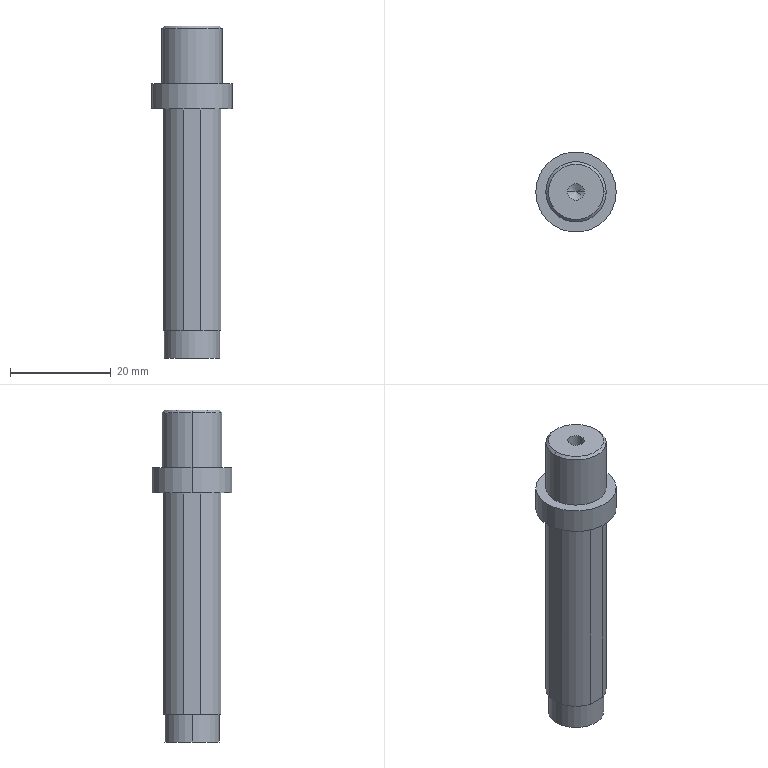Part | STEP file | Driven wheel shaft^Driven wheel assembly | 1 solid | 29 faces | box 16 x 16 x 66 mm | volume 7306 mm3 | cylinder 14 | plane 9 | cone 6 | commonest cylinder face diameters 12 x6 3.3 x2 5 x2 11 x2 16 x2
STEP:
#1=CARTESIAN_POINT('',(2.5,0.,-33.2));
#2=VERTEX_POINT('',#1);
#3=CARTESIAN_POINT('',(-2.5,0.,-33.2));
#4=VERTEX_POINT('',#3);
#5=CARTESIAN_POINT('',(0.,0.,-33.2));
#6=DIRECTION('',(0.,0.,-1.));
#7=DIRECTION('',(-1.,0.,0.));
#8=AXIS2_PLACEMENT_3D('',#5,#6,#7);
#9=CIRCLE('',#8,2.5);
#10=EDGE_CURVE('',#2,#4,#9,.T.);
#11=ORIENTED_EDGE('',*,*,#10,.F.);
#12=CARTESIAN_POINT('',(2.5,0.,-48.2));
#13=VERTEX_POINT('',#12);
#14=CARTESIAN_POINT('',(2.5,0.,-48.2));
#15=DIRECTION('',(0.,0.,-1.));
#16=VECTOR('',#15,1000.);
#17=LINE('',#14,#16);
#18=EDGE_CURVE('',#2,#13,#17,.T.);
#19=ORIENTED_EDGE('',*,*,#18,.T.);
#20=CARTESIAN_POINT('',(-2.5,0.,-48.2));
#21=VERTEX_POINT('',#20);
#22=CARTESIAN_POINT('',(0.,0.,-48.2));
#23=DIRECTION('',(0.,0.,-1.));
#24=DIRECTION('',(-1.,0.,0.));
#25=AXIS2_PLACEMENT_3D('',#22,#23,#24);
#26=CIRCLE('',#25,2.5);
#27=EDGE_CURVE('',#13,#21,#26,.T.);
#28=ORIENTED_EDGE('',*,*,#27,.T.);
#29=CARTESIAN_POINT('',(-2.5,0.,-48.2));
#30=DIRECTION('',(0.,0.,-1.));
#31=VECTOR('',#30,1000.);
#32=LINE('',#29,#31);
#33=EDGE_CURVE('',#4,#21,#32,.T.);
#34=ORIENTED_EDGE('',*,*,#33,.F.);
#35=EDGE_LOOP('',(#11,#19,#28,#34));
#36=FACE_OUTER_BOUND('',#35,.T.);
#37=CARTESIAN_POINT('',(0.,0.,-48.2));
#38=DIRECTION('',(0.,0.,-1.));
#39=DIRECTION('',(-1.,0.,0.));
#40=AXIS2_PLACEMENT_3D('',#37,#38,#39);
#41=CYLINDRICAL_SURFACE('',#40,2.5);
#42=ADVANCED_FACE('',(#36),#41,.F.);
#43=CARTESIAN_POINT('',(0.,0.,-31.698));
#44=VERTEX_POINT('',#43);
#45=CARTESIAN_POINT('',(-2.5,0.,-33.2));
#46=DIRECTION('',(-0.8572,0.,-0.515));
#47=VECTOR('',#46,1000.);
#48=LINE('',#45,#47);
#49=EDGE_CURVE('',#44,#4,#48,.T.);
#50=ORIENTED_EDGE('',*,*,#49,.F.);
#51=CARTESIAN_POINT('',(2.5,0.,-33.2));
#52=DIRECTION('',(0.8572,0.,-0.515));
#53=VECTOR('',#52,1000.);
#54=LINE('',#51,#53);
#55=EDGE_CURVE('',#44,#2,#54,.T.);
#56=ORIENTED_EDGE('',*,*,#55,.T.);
#57=ORIENTED_EDGE('',*,*,#10,.T.);
#58=EDGE_LOOP('',(#50,#56,#57));
#59=FACE_OUTER_BOUND('',#58,.T.);
#60=CARTESIAN_POINT('',(0.,0.,-33.2));
#61=DIRECTION('',(0.,0.,-1.));
#62=DIRECTION('',(-1.,0.,0.));
#63=AXIS2_PLACEMENT_3D('',#60,#61,#62);
#64=CONICAL_SURFACE('',#63,2.5,1.03);
#65=ADVANCED_FACE('',(#59),#64,.F.);
#66=CARTESIAN_POINT('',(-5.5,0.,-42.7));
#67=VERTEX_POINT('',#66);
#68=CARTESIAN_POINT('',(5.5,0.,-42.7));
#69=VERTEX_POINT('',#68);
#70=CARTESIAN_POINT('',(0.,0.,-42.7));
#71=DIRECTION('',(0.,0.,-1.));
#72=DIRECTION('',(-1.,0.,0.));
#73=AXIS2_PLACEMENT_3D('',#70,#71,#72);
#74=CIRCLE('',#73,5.5);
#75=EDGE_CURVE('',#67,#69,#74,.T.);
#76=ORIENTED_EDGE('',*,*,#75,.T.);
#77=CARTESIAN_POINT('',(5.5,0.,-48.2));
#78=VERTEX_POINT('',#77);
#79=CARTESIAN_POINT('',(5.5,0.,-42.7));
#80=DIRECTION('',(0.,0.,-1.));
#81=VECTOR('',#80,1000.);
#82=LINE('',#79,#81);
#83=EDGE_CURVE('',#69,#78,#82,.T.);
#84=ORIENTED_EDGE('',*,*,#83,.T.);
#85=CARTESIAN_POINT('',(-5.5,0.,-48.2));
#86=VERTEX_POINT('',#85);
#87=CARTESIAN_POINT('',(0.,0.,-48.2));
#88=DIRECTION('',(0.,0.,-1.));
#89=DIRECTION('',(-1.,0.,0.));
#90=AXIS2_PLACEMENT_3D('',#87,#88,#89);
#91=CIRCLE('',#90,5.5);
#92=EDGE_CURVE('',#86,#78,#91,.T.);
#93=ORIENTED_EDGE('',*,*,#92,.F.);
#94=CARTESIAN_POINT('',(-5.5,0.,-42.7));
#95=DIRECTION('',(0.,0.,-1.));
#96=VECTOR('',#95,1000.);
#97=LINE('',#94,#96);
#98=EDGE_CURVE('',#67,#86,#97,.T.);
#99=ORIENTED_EDGE('',*,*,#98,.F.);
#100=EDGE_LOOP('',(#76,#84,#93,#99));
#101=FACE_OUTER_BOUND('',#100,.T.);
#102=CARTESIAN_POINT('',(0.,0.,-42.7));
#103=DIRECTION('',(0.,0.,-1.));
#104=DIRECTION('',(-1.,0.,0.));
#105=AXIS2_PLACEMENT_3D('',#102,#103,#104);
#106=CYLINDRICAL_SURFACE('',#105,5.5);
#107=ADVANCED_FACE('',(#101),#106,.T.);
#108=CARTESIAN_POINT('',(-8.,0.,1.3));
#109=VERTEX_POINT('',#108);
#110=CARTESIAN_POINT('',(8.,0.,1.3));
#111=VERTEX_POINT('',#110);
#112=CARTESIAN_POINT('',(0.,0.,1.3));
#113=DIRECTION('',(0.,0.,-1.));
#114=DIRECTION('',(-1.,0.,0.));
#115=AXIS2_PLACEMENT_3D('',#112,#113,#114);
#116=CIRCLE('',#115,8.);
#117=EDGE_CURVE('',#109,#111,#116,.T.);
#118=ORIENTED_EDGE('',*,*,#117,.F.);
#119=CARTESIAN_POINT('',(-8.,0.,6.3));
#120=VERTEX_POINT('',#119);
#121=CARTESIAN_POINT('',(-8.,0.,1.3));
#122=DIRECTION('',(0.,0.,1.));
#123=VECTOR('',#122,1000.);
#124=LINE('',#121,#123);
#125=EDGE_CURVE('',#109,#120,#124,.T.);
#126=ORIENTED_EDGE('',*,*,#125,.T.);
#127=CARTESIAN_POINT('',(8.,0.,6.3));
#128=VERTEX_POINT('',#127);
#129=CARTESIAN_POINT('',(0.,0.,6.3));
#130=DIRECTION('',(0.,0.,-1.));
#131=DIRECTION('',(-1.,0.,0.));
#132=AXIS2_PLACEMENT_3D('',#129,#130,#131);
#133=CIRCLE('',#132,8.);
#134=EDGE_CURVE('',#120,#128,#133,.T.);
#135=ORIENTED_EDGE('',*,*,#134,.T.);
#136=CARTESIAN_POINT('',(8.,0.,1.3));
#137=DIRECTION('',(0.,0.,1.));
#138=VECTOR('',#137,1000.);
#139=LINE('',#136,#138);
#140=EDGE_CURVE('',#111,#128,#139,.T.);
#141=ORIENTED_EDGE('',*,*,#140,.F.);
#142=EDGE_LOOP('',(#118,#126,#135,#141));
#143=FACE_OUTER_BOUND('',#142,.T.);
#144=CARTESIAN_POINT('',(0.,0.,1.3));
#145=DIRECTION('',(0.,0.,1.));
#146=DIRECTION('',(1.,0.,0.));
#147=AXIS2_PLACEMENT_3D('',#144,#145,#146);
#148=CYLINDRICAL_SURFACE('',#147,8.);
#149=ADVANCED_FACE('',(#143),#148,.T.);
#150=CARTESIAN_POINT('',(-1.65,0.,7.7));
#151=VERTEX_POINT('',#150);
#152=CARTESIAN_POINT('',(1.65,0.,7.7));
#153=VERTEX_POINT('',#152);
#154=CARTESIAN_POINT('',(0.,0.,7.7));
#155=DIRECTION('',(0.,0.,1.));
#156=DIRECTION('',(1.,0.,0.));
#157=AXIS2_PLACEMENT_3D('',#154,#155,#156);
#158=CIRCLE('',#157,1.65);
#159=EDGE_CURVE('',#151,#153,#158,.T.);
#160=ORIENTED_EDGE('',*,*,#159,.F.);
#161=CARTESIAN_POINT('',(-1.65,0.,17.8));
#162=VERTEX_POINT('',#161);
#163=CARTESIAN_POINT('',(-1.65,0.,17.8));
#164=DIRECTION('',(0.,0.,1.));
#165=VECTOR('',#164,1000.);
#166=LINE('',#163,#165);
#167=EDGE_CURVE('',#151,#162,#166,.T.);
#168=ORIENTED_EDGE('',*,*,#167,.T.);
#169=CARTESIAN_POINT('',(1.65,0.,17.8));
#170=VERTEX_POINT('',#169);
#171=CARTESIAN_POINT('',(0.,0.,17.8));
#172=DIRECTION('',(0.,0.,1.));
#173=DIRECTION('',(1.,0.,0.));
#174=AXIS2_PLACEMENT_3D('',#171,#172,#173);
#175=CIRCLE('',#174,1.65);
#176=EDGE_CURVE('',#162,#170,#175,.T.);
#177=ORIENTED_EDGE('',*,*,#176,.T.);
#178=CARTESIAN_POINT('',(1.65,0.,17.8));
#179=DIRECTION('',(0.,0.,1.));
#180=VECTOR('',#179,1000.);
#181=LINE('',#178,#180);
#182=EDGE_CURVE('',#153,#170,#181,.T.);
#183=ORIENTED_EDGE('',*,*,#182,.F.);
#184=EDGE_LOOP('',(#160,#168,#177,#183));
#185=FACE_OUTER_BOUND('',#184,.T.);
#186=CARTESIAN_POINT('',(0.,0.,17.8));
#187=DIRECTION('',(0.,0.,1.));
#188=DIRECTION('',(1.,0.,0.));
#189=AXIS2_PLACEMENT_3D('',#186,#187,#188);
#190=CYLINDRICAL_SURFACE('',#189,1.65);
#191=ADVANCED_FACE('',(#185),#190,.F.);
#192=CARTESIAN_POINT('',(0.,0.,6.709));
#193=VERTEX_POINT('',#192);
#194=CARTESIAN_POINT('',(1.65,0.,7.7));
#195=DIRECTION('',(0.8572,0.,0.515));
#196=VECTOR('',#195,1000.);
#197=LINE('',#194,#196);
#198=EDGE_CURVE('',#193,#153,#197,.T.);
#199=ORIENTED_EDGE('',*,*,#198,.F.);
#200=CARTESIAN_POINT('',(-1.65,0.,7.7));
#201=DIRECTION('',(-0.8572,0.,0.515));
#202=VECTOR('',#201,1000.);
#203=LINE('',#200,#202);
#204=EDGE_CURVE('',#193,#151,#203,.T.);
#205=ORIENTED_EDGE('',*,*,#204,.T.);
#206=ORIENTED_EDGE('',*,*,#159,.T.);
#207=EDGE_LOOP('',(#199,#205,#206));
#208=FACE_OUTER_BOUND('',#207,.T.);
#209=CARTESIAN_POINT('',(0.,0.,7.7));
#210=DIRECTION('',(0.,0.,1.));
#211=DIRECTION('',(1.,0.,0.));
#212=AXIS2_PLACEMENT_3D('',#209,#210,#211);
#213=CONICAL_SURFACE('',#212,1.65,1.03);
#214=ADVANCED_FACE('',(#208),#213,.F.);
#215=CARTESIAN_POINT('',(5.5,0.,17.8));
#216=VERTEX_POINT('',#215);
#217=CARTESIAN_POINT('',(-5.5,0.,17.8));
#218=VERTEX_POINT('',#217);
#219=CARTESIAN_POINT('',(0.,0.,17.8));
#220=DIRECTION('',(0.,0.,1.));
#221=DIRECTION('',(1.,0.,0.));
#222=AXIS2_PLACEMENT_3D('',#219,#220,#221);
#223=CIRCLE('',#222,5.5);
#224=EDGE_CURVE('',#216,#218,#223,.T.);
#225=ORIENTED_EDGE('',*,*,#224,.F.);
#226=CARTESIAN_POINT('',(6.,0.,17.3));
#227=VERTEX_POINT('',#226);
#228=CARTESIAN_POINT('',(5.5,0.,17.8));
#229=DIRECTION('',(0.7071,0.,-0.7071));
#230=VECTOR('',#229,1000.);
#231=LINE('',#228,#230);
#232=EDGE_CURVE('',#216,#227,#231,.T.);
#233=ORIENTED_EDGE('',*,*,#232,.T.);
#234=CARTESIAN_POINT('',(-6.,0.,17.3));
#235=VERTEX_POINT('',#234);
#236=CARTESIAN_POINT('',(0.,0.,17.3));
#237=DIRECTION('',(0.,0.,-1.));
#238=DIRECTION('',(1.,0.,0.));
#239=AXIS2_PLACEMENT_3D('',#236,#237,#238);
#240=CIRCLE('',#239,6.);
#241=EDGE_CURVE('',#235,#227,#240,.T.);
#242=ORIENTED_EDGE('',*,*,#241,.F.);
#243=CARTESIAN_POINT('',(-5.5,0.,17.8));
#244=DIRECTION('',(-0.7071,0.,-0.7071));
#245=VECTOR('',#244,1000.);
#246=LINE('',#243,#245);
#247=EDGE_CURVE('',#218,#235,#246,.T.);
#248=ORIENTED_EDGE('',*,*,#247,.F.);
#249=EDGE_LOOP('',(#225,#233,#242,#248));
#250=FACE_OUTER_BOUND('',#249,.T.);
#251=CARTESIAN_POINT('',(0.,0.,17.8));
#252=DIRECTION('',(0.,0.,-1.));
#253=DIRECTION('',(-1.,0.,0.));
#254=AXIS2_PLACEMENT_3D('',#251,#252,#253);
#255=CONICAL_SURFACE('',#254,5.5,0.7854);
#256=ADVANCED_FACE('',(#250),#255,.T.);
#257=CARTESIAN_POINT('',(6.,0.,6.3));
#258=VERTEX_POINT('',#257);
#259=CARTESIAN_POINT('',(-6.,0.,6.3));
#260=VERTEX_POINT('',#259);
#261=CARTESIAN_POINT('',(0.,0.,6.3));
#262=DIRECTION('',(0.,0.,1.));
#263=DIRECTION('',(-1.,0.,0.));
#264=AXIS2_PLACEMENT_3D('',#261,#262,#263);
#265=CIRCLE('',#264,6.);
#266=EDGE_CURVE('',#258,#260,#265,.T.);
#267=ORIENTED_EDGE('',*,*,#266,.T.);
#268=CARTESIAN_POINT('',(-6.,0.,-48.2));
#269=DIRECTION('',(0.,0.,1.));
#270=VECTOR('',#269,1000.);
#271=LINE('',#268,#270);
#272=EDGE_CURVE('',#260,#235,#271,.T.);
#273=ORIENTED_EDGE('',*,*,#272,.T.);
#274=ORIENTED_EDGE('',*,*,#241,.T.);
#275=CARTESIAN_POINT('',(6.,0.,-48.2));
#276=DIRECTION('',(0.,0.,1.));
#277=VECTOR('',#276,1000.);
#278=LINE('',#275,#277);
#279=EDGE_CURVE('',#258,#227,#278,.T.);
#280=ORIENTED_EDGE('',*,*,#279,.F.);
#281=EDGE_LOOP('',(#267,#273,#274,#280));
#282=FACE_OUTER_BOUND('',#281,.T.);
#283=CARTESIAN_POINT('',(0.,0.,-48.2));
#284=DIRECTION('',(0.,0.,1.));
#285=DIRECTION('',(1.,0.,0.));
#286=AXIS2_PLACEMENT_3D('',#283,#284,#285);
#287=CYLINDRICAL_SURFACE('',#286,6.);
#288=ADVANCED_FACE('',(#282),#287,.T.);
#289=CARTESIAN_POINT('',(5.75,1.714,-42.7));
#290=VERTEX_POINT('',#289);
#291=CARTESIAN_POINT('',(1.714,5.75,-42.7));
#292=VERTEX_POINT('',#291);
#293=CARTESIAN_POINT('',(0.,0.,-42.7));
#294=DIRECTION('',(0.,0.,1.));
#295=DIRECTION('',(-1.,0.,0.));
#296=AXIS2_PLACEMENT_3D('',#293,#294,#295);
#297=CIRCLE('',#296,6.);
#298=EDGE_CURVE('',#290,#292,#297,.T.);
#299=ORIENTED_EDGE('',*,*,#298,.T.);
#300=CARTESIAN_POINT('',(1.714,5.75,1.3));
#301=VERTEX_POINT('',#300);
#302=CARTESIAN_POINT('',(1.714,5.75,-48.2));
#303=DIRECTION('',(0.,0.,1.));
#304=VECTOR('',#303,1000.);
#305=LINE('',#302,#304);
#306=EDGE_CURVE('',#292,#301,#305,.T.);
#307=ORIENTED_EDGE('',*,*,#306,.T.);
#308=CARTESIAN_POINT('',(5.75,1.714,1.3));
#309=VERTEX_POINT('',#308);
#310=CARTESIAN_POINT('',(0.,0.,1.3));
#311=DIRECTION('',(0.,0.,1.));
#312=DIRECTION('',(-1.,0.,0.));
#313=AXIS2_PLACEMENT_3D('',#310,#311,#312);
#314=CIRCLE('',#313,6.);
#315=EDGE_CURVE('',#309,#301,#314,.T.);
#316=ORIENTED_EDGE('',*,*,#315,.F.);
#317=CARTESIAN_POINT('',(5.75,1.714,-48.2));
#318=DIRECTION('',(0.,0.,-1.));
#319=VECTOR('',#318,1000.);
#320=LINE('',#317,#319);
#321=EDGE_CURVE('',#309,#290,#320,.T.);
#322=ORIENTED_EDGE('',*,*,#321,.T.);
#323=EDGE_LOOP('',(#299,#307,#316,#322));
#324=FACE_OUTER_BOUND('',#323,.T.);
#325=CARTESIAN_POINT('',(0.,0.,-48.2));
#326=DIRECTION('',(0.,0.,1.));
#327=DIRECTION('',(1.,0.,0.));
#328=AXIS2_PLACEMENT_3D('',#325,#326,#327);
#329=CYLINDRICAL_SURFACE('',#328,6.);
#330=ADVANCED_FACE('',(#324),#329,.T.);
#331=CARTESIAN_POINT('',(-5.75,-1.714,-42.7));
#332=VERTEX_POINT('',#331);
#333=CARTESIAN_POINT('',(-1.714,-5.75,-42.7));
#334=VERTEX_POINT('',#333);
#335=CARTESIAN_POINT('',(0.,0.,-42.7));
#336=DIRECTION('',(0.,0.,1.));
#337=DIRECTION('',(-1.,0.,0.));
#338=AXIS2_PLACEMENT_3D('',#335,#336,#337);
#339=CIRCLE('',#338,6.);
#340=EDGE_CURVE('',#332,#334,#339,.T.);
#341=ORIENTED_EDGE('',*,*,#340,.T.);
#342=CARTESIAN_POINT('',(-1.714,-5.75,1.3));
#343=VERTEX_POINT('',#342);
#344=CARTESIAN_POINT('',(-1.714,-5.75,-48.2));
#345=DIRECTION('',(0.,0.,1.));
#346=VECTOR('',#345,1000.);
#347=LINE('',#344,#346);
#348=EDGE_CURVE('',#334,#343,#347,.T.);
#349=ORIENTED_EDGE('',*,*,#348,.T.);
#350=CARTESIAN_POINT('',(-5.75,-1.714,1.3));
#351=VERTEX_POINT('',#350);
#352=CARTESIAN_POINT('',(0.,0.,1.3));
#353=DIRECTION('',(0.,0.,1.));
#354=DIRECTION('',(-1.,0.,0.));
#355=AXIS2_PLACEMENT_3D('',#352,#353,#354);
#356=CIRCLE('',#355,6.);
#357=EDGE_CURVE('',#351,#343,#356,.T.);
#358=ORIENTED_EDGE('',*,*,#357,.F.);
#359=CARTESIAN_POINT('',(-5.75,-1.714,-48.2));
#360=DIRECTION('',(0.,0.,-1.));
#361=VECTOR('',#360,1000.);
#362=LINE('',#359,#361);
#363=EDGE_CURVE('',#351,#332,#362,.T.);
#364=ORIENTED_EDGE('',*,*,#363,.T.);
#365=EDGE_LOOP('',(#341,#349,#358,#364));
#366=FACE_OUTER_BOUND('',#365,.T.);
#367=CARTESIAN_POINT('',(0.,0.,-48.2));
#368=DIRECTION('',(0.,0.,1.));
#369=DIRECTION('',(1.,0.,0.));
#370=AXIS2_PLACEMENT_3D('',#367,#368,#369);
#371=CYLINDRICAL_SURFACE('',#370,6.);
#372=ADVANCED_FACE('',(#366),#371,.T.);
#373=CARTESIAN_POINT('',(5.75,-1.714,-42.7));
#374=VERTEX_POINT('',#373);
#375=CARTESIAN_POINT('',(5.75,-1.714,1.3));
#376=VERTEX_POINT('',#375);
#377=CARTESIAN_POINT('',(5.75,-1.714,-48.2));
#378=DIRECTION('',(0.,0.,1.));
#379=VECTOR('',#378,1000.);
#380=LINE('',#377,#379);
#381=EDGE_CURVE('',#374,#376,#380,.T.);
#382=ORIENTED_EDGE('',*,*,#381,.F.);
#383=CARTESIAN_POINT('',(5.75,15.529,-42.7));
#384=DIRECTION('',(0.,1.,0.));
#385=VECTOR('',#384,1000.);
#386=LINE('',#383,#385);
#387=EDGE_CURVE('',#374,#290,#386,.T.);
#388=ORIENTED_EDGE('',*,*,#387,.T.);
#389=ORIENTED_EDGE('',*,*,#321,.F.);
#390=CARTESIAN_POINT('',(5.75,15.529,1.3));
#391=DIRECTION('',(0.,1.,0.));
#392=VECTOR('',#391,1000.);
#393=LINE('',#390,#392);
#394=EDGE_CURVE('',#376,#309,#393,.T.);
#395=ORIENTED_EDGE('',*,*,#394,.F.);
#396=EDGE_LOOP('',(#382,#388,#389,#395));
#397=FACE_OUTER_BOUND('',#396,.T.);
#398=CARTESIAN_POINT('',(5.75,15.529,36.586));
#399=DIRECTION('',(1.,0.,0.));
#400=DIRECTION('',(0.,0.,-1.));
#401=AXIS2_PLACEMENT_3D('',#398,#399,#400);
#402=PLANE('',#401);
#403=ADVANCED_FACE('',(#397),#402,.T.);
#404=CARTESIAN_POINT('',(-5.75,1.714,-42.7));
#405=VERTEX_POINT('',#404);
#406=CARTESIAN_POINT('',(-5.75,1.714,1.3));
#407=VERTEX_POINT('',#406);
#408=CARTESIAN_POINT('',(-5.75,1.714,-48.2));
#409=DIRECTION('',(0.,0.,1.));
#410=VECTOR('',#409,1000.);
#411=LINE('',#408,#410);
#412=EDGE_CURVE('',#405,#407,#411,.T.);
#413=ORIENTED_EDGE('',*,*,#412,.F.);
#414=CARTESIAN_POINT('',(-5.75,15.529,-42.7));
#415=DIRECTION('',(0.,-1.,0.));
#416=VECTOR('',#415,1000.);
#417=LINE('',#414,#416);
#418=EDGE_CURVE('',#405,#332,#417,.T.);
#419=ORIENTED_EDGE('',*,*,#418,.T.);
#420=ORIENTED_EDGE('',*,*,#363,.F.);
#421=CARTESIAN_POINT('',(-5.75,15.529,1.3));
#422=DIRECTION('',(0.,-1.,0.));
#423=VECTOR('',#422,1000.);
#424=LINE('',#421,#423);
#425=EDGE_CURVE('',#407,#351,#424,.T.);
#426=ORIENTED_EDGE('',*,*,#425,.F.);
#427=EDGE_LOOP('',(#413,#419,#420,#426));
#428=FACE_OUTER_BOUND('',#427,.T.);
#429=CARTESIAN_POINT('',(-5.75,15.529,36.586));
#430=DIRECTION('',(-1.,0.,0.));
#431=DIRECTION('',(0.,0.,1.));
#432=AXIS2_PLACEMENT_3D('',#429,#430,#431);
#433=PLANE('',#432);
#434=ADVANCED_FACE('',(#428),#433,.T.);
#435=CARTESIAN_POINT('',(-1.714,5.75,-42.7));
#436=VERTEX_POINT('',#435);
#437=CARTESIAN_POINT('',(0.,0.,-42.7));
#438=DIRECTION('',(0.,0.,1.));
#439=DIRECTION('',(-1.,0.,0.));
#440=AXIS2_PLACEMENT_3D('',#437,#438,#439);
#441=CIRCLE('',#440,6.);
#442=EDGE_CURVE('',#436,#405,#441,.T.);
#443=ORIENTED_EDGE('',*,*,#442,.T.);
#444=ORIENTED_EDGE('',*,*,#412,.T.);
#445=CARTESIAN_POINT('',(-1.714,5.75,1.3));
#446=VERTEX_POINT('',#445);
#447=CARTESIAN_POINT('',(0.,0.,1.3));
#448=DIRECTION('',(0.,0.,1.));
#449=DIRECTION('',(-1.,0.,0.));
#450=AXIS2_PLACEMENT_3D('',#447,#448,#449);
#451=CIRCLE('',#450,6.);
#452=EDGE_CURVE('',#446,#407,#451,.T.);
#453=ORIENTED_EDGE('',*,*,#452,.F.);
#454=CARTESIAN_POINT('',(-1.714,5.75,-48.2));
#455=DIRECTION('',(0.,0.,-1.));
#456=VECTOR('',#455,1000.);
#457=LINE('',#454,#456);
#458=EDGE_CURVE('',#446,#436,#457,.T.);
#459=ORIENTED_EDGE('',*,*,#458,.T.);
#460=EDGE_LOOP('',(#443,#444,#453,#459));
#461=FACE_OUTER_BOUND('',#460,.T.);
#462=CARTESIAN_POINT('',(0.,0.,-48.2));
#463=DIRECTION('',(0.,0.,1.));
#464=DIRECTION('',(1.,0.,0.));
#465=AXIS2_PLACEMENT_3D('',#462,#463,#464);
#466=CYLINDRICAL_SURFACE('',#465,6.);
#467=ADVANCED_FACE('',(#461),#466,.T.);
#468=CARTESIAN_POINT('',(1.714,-5.75,-42.7));
#469=VERTEX_POINT('',#468);
#470=CARTESIAN_POINT('',(0.,0.,-42.7));
#471=DIRECTION('',(0.,0.,1.));
#472=DIRECTION('',(-1.,0.,0.));
#473=AXIS2_PLACEMENT_3D('',#470,#471,#472);
#474=CIRCLE('',#473,6.);
#475=EDGE_CURVE('',#469,#374,#474,.T.);
#476=ORIENTED_EDGE('',*,*,#475,.T.);
#477=ORIENTED_EDGE('',*,*,#381,.T.);
#478=CARTESIAN_POINT('',(1.714,-5.75,1.3));
#479=VERTEX_POINT('',#478);
#480=CARTESIAN_POINT('',(0.,0.,1.3));
#481=DIRECTION('',(0.,0.,1.));
#482=DIRECTION('',(-1.,0.,0.));
#483=AXIS2_PLACEMENT_3D('',#480,#481,#482);
#484=CIRCLE('',#483,6.);
#485=EDGE_CURVE('',#479,#376,#484,.T.);
#486=ORIENTED_EDGE('',*,*,#485,.F.);
#487=CARTESIAN_POINT('',(1.714,-5.75,-48.2));
#488=DIRECTION('',(0.,0.,-1.));
#489=VECTOR('',#488,1000.);
#490=LINE('',#487,#489);
#491=EDGE_CURVE('',#479,#469,#490,.T.);
#492=ORIENTED_EDGE('',*,*,#491,.T.);
#493=EDGE_LOOP('',(#476,#477,#486,#492));
#494=FACE_OUTER_BOUND('',#493,.T.);
#495=CARTESIAN_POINT('',(0.,0.,-48.2));
#496=DIRECTION('',(0.,0.,1.));
#497=DIRECTION('',(1.,0.,0.));
#498=AXIS2_PLACEMENT_3D('',#495,#496,#497);
#499=CYLINDRICAL_SURFACE('',#498,6.);
#500=ADVANCED_FACE('',(#494),#499,.T.);
#501=ORIENTED_EDGE('',*,*,#306,.F.);
#502=CARTESIAN_POINT('',(15.529,5.75,-42.7));
#503=DIRECTION('',(-1.,0.,0.));
#504=VECTOR('',#503,1000.);
#505=LINE('',#502,#504);
#506=EDGE_CURVE('',#292,#436,#505,.T.);
#507=ORIENTED_EDGE('',*,*,#506,.T.);
#508=ORIENTED_EDGE('',*,*,#458,.F.);
#509=CARTESIAN_POINT('',(15.529,5.75,1.3));
#510=DIRECTION('',(-1.,0.,0.));
#511=VECTOR('',#510,1000.);
#512=LINE('',#509,#511);
#513=EDGE_CURVE('',#301,#446,#512,.T.);
#514=ORIENTED_EDGE('',*,*,#513,.F.);
#515=EDGE_LOOP('',(#501,#507,#508,#514));
#516=FACE_OUTER_BOUND('',#515,.T.);
#517=CARTESIAN_POINT('',(15.529,5.75,36.586));
#518=DIRECTION('',(0.,1.,0.));
#519=DIRECTION('',(0.,0.,1.));
#520=AXIS2_PLACEMENT_3D('',#517,#518,#519);
#521=PLANE('',#520);
#522=ADVANCED_FACE('',(#516),#521,.T.);
#523=ORIENTED_EDGE('',*,*,#348,.F.);
#524=CARTESIAN_POINT('',(15.529,-5.75,-42.7));
#525=DIRECTION('',(1.,0.,0.));
#526=VECTOR('',#525,1000.);
#527=LINE('',#524,#526);
#528=EDGE_CURVE('',#334,#469,#527,.T.);
#529=ORIENTED_EDGE('',*,*,#528,.T.);
#530=ORIENTED_EDGE('',*,*,#491,.F.);
#531=CARTESIAN_POINT('',(15.529,-5.75,1.3));
#532=DIRECTION('',(1.,0.,0.));
#533=VECTOR('',#532,1000.);
#534=LINE('',#531,#533);
#535=EDGE_CURVE('',#343,#479,#534,.T.);
#536=ORIENTED_EDGE('',*,*,#535,.F.);
#537=EDGE_LOOP('',(#523,#529,#530,#536));
#538=FACE_OUTER_BOUND('',#537,.T.);
#539=CARTESIAN_POINT('',(15.529,-5.75,36.586));
#540=DIRECTION('',(0.,-1.,0.));
#541=DIRECTION('',(0.,0.,-1.));
#542=AXIS2_PLACEMENT_3D('',#539,#540,#541);
#543=PLANE('',#542);
#544=ADVANCED_FACE('',(#538),#543,.T.);
#545=ORIENTED_EDGE('',*,*,#272,.F.);
#546=CARTESIAN_POINT('',(0.,0.,6.3));
#547=DIRECTION('',(0.,0.,1.));
#548=DIRECTION('',(-1.,0.,0.));
#549=AXIS2_PLACEMENT_3D('',#546,#547,#548);
#550=CIRCLE('',#549,6.);
#551=EDGE_CURVE('',#260,#258,#550,.T.);
#552=ORIENTED_EDGE('',*,*,#551,.T.);
#553=ORIENTED_EDGE('',*,*,#279,.T.);
#554=CARTESIAN_POINT('',(0.,0.,17.3));
#555=DIRECTION('',(0.,0.,-1.));
#556=DIRECTION('',(1.,0.,0.));
#557=AXIS2_PLACEMENT_3D('',#554,#555,#556);
#558=CIRCLE('',#557,6.);
#559=EDGE_CURVE('',#227,#235,#558,.T.);
#560=ORIENTED_EDGE('',*,*,#559,.T.);
#561=EDGE_LOOP('',(#545,#552,#553,#560));
#562=FACE_OUTER_BOUND('',#561,.T.);
#563=CARTESIAN_POINT('',(0.,0.,-48.2));
#564=DIRECTION('',(0.,0.,1.));
#565=DIRECTION('',(1.,0.,0.));
#566=AXIS2_PLACEMENT_3D('',#563,#564,#565);
#567=CYLINDRICAL_SURFACE('',#566,6.);
#568=ADVANCED_FACE('',(#562),#567,.T.);
#569=CARTESIAN_POINT('',(0.,0.,17.8));
#570=DIRECTION('',(0.,0.,1.));
#571=DIRECTION('',(1.,0.,0.));
#572=AXIS2_PLACEMENT_3D('',#569,#570,#571);
#573=CIRCLE('',#572,1.65);
#574=EDGE_CURVE('',#170,#162,#573,.T.);
#575=ORIENTED_EDGE('',*,*,#574,.F.);
#576=ORIENTED_EDGE('',*,*,#176,.F.);
#577=EDGE_LOOP('',(#575,#576));
#578=FACE_BOUND('',#577,.T.);
#579=CARTESIAN_POINT('',(0.,0.,17.8));
#580=DIRECTION('',(0.,0.,1.));
#581=DIRECTION('',(1.,0.,0.));
#582=AXIS2_PLACEMENT_3D('',#579,#580,#581);
#583=CIRCLE('',#582,5.5);
#584=EDGE_CURVE('',#218,#216,#583,.T.);
#585=ORIENTED_EDGE('',*,*,#584,.T.);
#586=ORIENTED_EDGE('',*,*,#224,.T.);
#587=EDGE_LOOP('',(#585,#586));
#588=FACE_OUTER_BOUND('',#587,.T.);
#589=CARTESIAN_POINT('',(0.,0.,17.8));
#590=DIRECTION('',(0.,0.,1.));
#591=DIRECTION('',(1.,0.,0.));
#592=AXIS2_PLACEMENT_3D('',#589,#590,#591);
#593=PLANE('',#592);
#594=ADVANCED_FACE('',(#578,#588),#593,.T.);
#595=ORIENTED_EDGE('',*,*,#232,.F.);
#596=ORIENTED_EDGE('',*,*,#584,.F.);
#597=ORIENTED_EDGE('',*,*,#247,.T.);
#598=ORIENTED_EDGE('',*,*,#559,.F.);
#599=EDGE_LOOP('',(#595,#596,#597,#598));
#600=FACE_OUTER_BOUND('',#599,.T.);
#601=CARTESIAN_POINT('',(0.,0.,17.8));
#602=DIRECTION('',(0.,0.,-1.));
#603=DIRECTION('',(-1.,0.,0.));
#604=AXIS2_PLACEMENT_3D('',#601,#602,#603);
#605=CONICAL_SURFACE('',#604,5.5,0.7854);
#606=ADVANCED_FACE('',(#600),#605,.T.);
#607=ORIENTED_EDGE('',*,*,#204,.F.);
#608=ORIENTED_EDGE('',*,*,#198,.T.);
#609=CARTESIAN_POINT('',(0.,0.,7.7));
#610=DIRECTION('',(0.,0.,1.));
#611=DIRECTION('',(1.,0.,0.));
#612=AXIS2_PLACEMENT_3D('',#609,#610,#611);
#613=CIRCLE('',#612,1.65);
#614=EDGE_CURVE('',#153,#151,#613,.T.);
#615=ORIENTED_EDGE('',*,*,#614,.T.);
#616=EDGE_LOOP('',(#607,#608,#615));
#617=FACE_OUTER_BOUND('',#616,.T.);
#618=CARTESIAN_POINT('',(0.,0.,7.7));
#619=DIRECTION('',(0.,0.,1.));
#620=DIRECTION('',(1.,0.,0.));
#621=AXIS2_PLACEMENT_3D('',#618,#619,#620);
#622=CONICAL_SURFACE('',#621,1.65,1.03);
#623=ADVANCED_FACE('',(#617),#622,.F.);
#624=ORIENTED_EDGE('',*,*,#167,.F.);
#625=ORIENTED_EDGE('',*,*,#614,.F.);
#626=ORIENTED_EDGE('',*,*,#182,.T.);
#627=ORIENTED_EDGE('',*,*,#574,.T.);
#628=EDGE_LOOP('',(#624,#625,#626,#627));
#629=FACE_OUTER_BOUND('',#628,.T.);
#630=CARTESIAN_POINT('',(0.,0.,17.8));
#631=DIRECTION('',(0.,0.,1.));
#632=DIRECTION('',(1.,0.,0.));
#633=AXIS2_PLACEMENT_3D('',#630,#631,#632);
#634=CYLINDRICAL_SURFACE('',#633,1.65);
#635=ADVANCED_FACE('',(#629),#634,.F.);
#636=ORIENTED_EDGE('',*,*,#125,.F.);
#637=CARTESIAN_POINT('',(0.,0.,1.3));
#638=DIRECTION('',(0.,0.,-1.));
#639=DIRECTION('',(-1.,0.,0.));
#640=AXIS2_PLACEMENT_3D('',#637,#638,#639);
#641=CIRCLE('',#640,8.);
#642=EDGE_CURVE('',#111,#109,#641,.T.);
#643=ORIENTED_EDGE('',*,*,#642,.F.);
#644=ORIENTED_EDGE('',*,*,#140,.T.);
#645=CARTESIAN_POINT('',(0.,0.,6.3));
#646=DIRECTION('',(0.,0.,-1.));
#647=DIRECTION('',(-1.,0.,0.));
#648=AXIS2_PLACEMENT_3D('',#645,#646,#647);
#649=CIRCLE('',#648,8.);
#650=EDGE_CURVE('',#128,#120,#649,.T.);
#651=ORIENTED_EDGE('',*,*,#650,.T.);
#652=EDGE_LOOP('',(#636,#643,#644,#651));
#653=FACE_OUTER_BOUND('',#652,.T.);
#654=CARTESIAN_POINT('',(0.,0.,1.3));
#655=DIRECTION('',(0.,0.,1.));
#656=DIRECTION('',(1.,0.,0.));
#657=AXIS2_PLACEMENT_3D('',#654,#655,#656);
#658=CYLINDRICAL_SURFACE('',#657,8.);
#659=ADVANCED_FACE('',(#653),#658,.T.);
#660=ORIENTED_EDGE('',*,*,#485,.T.);
#661=ORIENTED_EDGE('',*,*,#394,.T.);
#662=ORIENTED_EDGE('',*,*,#315,.T.);
#663=ORIENTED_EDGE('',*,*,#513,.T.);
#664=ORIENTED_EDGE('',*,*,#452,.T.);
#665=ORIENTED_EDGE('',*,*,#425,.T.);
#666=ORIENTED_EDGE('',*,*,#357,.T.);
#667=ORIENTED_EDGE('',*,*,#535,.T.);
#668=EDGE_LOOP('',(#660,#661,#662,#663,#664,#665,#666,#667));
#669=FACE_BOUND('',#668,.T.);
#670=ORIENTED_EDGE('',*,*,#642,.T.);
#671=ORIENTED_EDGE('',*,*,#117,.T.);
#672=EDGE_LOOP('',(#670,#671));
#673=FACE_OUTER_BOUND('',#672,.T.);
#674=CARTESIAN_POINT('',(0.,0.,1.3));
#675=DIRECTION('',(0.,0.,-1.));
#676=DIRECTION('',(-1.,0.,0.));
#677=AXIS2_PLACEMENT_3D('',#674,#675,#676);
#678=PLANE('',#677);
#679=ADVANCED_FACE('',(#669,#673),#678,.T.);
#680=ORIENTED_EDGE('',*,*,#266,.F.);
#681=ORIENTED_EDGE('',*,*,#551,.F.);
#682=EDGE_LOOP('',(#680,#681));
#683=FACE_BOUND('',#682,.T.);
#684=ORIENTED_EDGE('',*,*,#650,.F.);
#685=ORIENTED_EDGE('',*,*,#134,.F.);
#686=EDGE_LOOP('',(#684,#685));
#687=FACE_OUTER_BOUND('',#686,.T.);
#688=CARTESIAN_POINT('',(0.,0.,6.3));
#689=DIRECTION('',(0.,0.,-1.));
#690=DIRECTION('',(-1.,0.,0.));
#691=AXIS2_PLACEMENT_3D('',#688,#689,#690);
#692=PLANE('',#691);
#693=ADVANCED_FACE('',(#683,#687),#692,.F.);
#694=ORIENTED_EDGE('',*,*,#442,.F.);
#695=ORIENTED_EDGE('',*,*,#506,.F.);
#696=ORIENTED_EDGE('',*,*,#298,.F.);
#697=ORIENTED_EDGE('',*,*,#387,.F.);
#698=ORIENTED_EDGE('',*,*,#475,.F.);
#699=ORIENTED_EDGE('',*,*,#528,.F.);
#700=ORIENTED_EDGE('',*,*,#340,.F.);
#701=ORIENTED_EDGE('',*,*,#418,.F.);
#702=EDGE_LOOP('',(#694,#695,#696,#697,#698,#699,#700,#701));
#703=FACE_OUTER_BOUND('',#702,.T.);
#704=ORIENTED_EDGE('',*,*,#75,.F.);
#705=CARTESIAN_POINT('',(0.,0.,-42.7));
#706=DIRECTION('',(0.,0.,-1.));
#707=DIRECTION('',(-1.,0.,0.));
#708=AXIS2_PLACEMENT_3D('',#705,#706,#707);
#709=CIRCLE('',#708,5.5);
#710=EDGE_CURVE('',#69,#67,#709,.T.);
#711=ORIENTED_EDGE('',*,*,#710,.F.);
#712=EDGE_LOOP('',(#704,#711));
#713=FACE_BOUND('',#712,.T.);
#714=CARTESIAN_POINT('',(0.,0.,-42.7));
#715=DIRECTION('',(0.,0.,-1.));
#716=DIRECTION('',(-1.,0.,0.));
#717=AXIS2_PLACEMENT_3D('',#714,#715,#716);
#718=PLANE('',#717);
#719=ADVANCED_FACE('',(#703,#713),#718,.T.);
#720=ORIENTED_EDGE('',*,*,#83,.F.);
#721=ORIENTED_EDGE('',*,*,#710,.T.);
#722=ORIENTED_EDGE('',*,*,#98,.T.);
#723=CARTESIAN_POINT('',(0.,0.,-48.2));
#724=DIRECTION('',(0.,0.,-1.));
#725=DIRECTION('',(-1.,0.,0.));
#726=AXIS2_PLACEMENT_3D('',#723,#724,#725);
#727=CIRCLE('',#726,5.5);
#728=EDGE_CURVE('',#78,#86,#727,.T.);
#729=ORIENTED_EDGE('',*,*,#728,.F.);
#730=EDGE_LOOP('',(#720,#721,#722,#729));
#731=FACE_OUTER_BOUND('',#730,.T.);
#732=CARTESIAN_POINT('',(0.,0.,-42.7));
#733=DIRECTION('',(0.,0.,-1.));
#734=DIRECTION('',(-1.,0.,0.));
#735=AXIS2_PLACEMENT_3D('',#732,#733,#734);
#736=CYLINDRICAL_SURFACE('',#735,5.5);
#737=ADVANCED_FACE('',(#731),#736,.T.);
#738=CARTESIAN_POINT('',(0.,0.,-48.2));
#739=DIRECTION('',(0.,0.,-1.));
#740=DIRECTION('',(-1.,0.,0.));
#741=AXIS2_PLACEMENT_3D('',#738,#739,#740);
#742=CIRCLE('',#741,2.5);
#743=EDGE_CURVE('',#21,#13,#742,.T.);
#744=ORIENTED_EDGE('',*,*,#743,.F.);
#745=ORIENTED_EDGE('',*,*,#27,.F.);
#746=EDGE_LOOP('',(#744,#745));
#747=FACE_BOUND('',#746,.T.);
#748=ORIENTED_EDGE('',*,*,#92,.T.);
#749=ORIENTED_EDGE('',*,*,#728,.T.);
#750=EDGE_LOOP('',(#748,#749));
#751=FACE_OUTER_BOUND('',#750,.T.);
#752=CARTESIAN_POINT('',(0.,0.,-48.2));
#753=DIRECTION('',(0.,0.,1.));
#754=DIRECTION('',(1.,0.,0.));
#755=AXIS2_PLACEMENT_3D('',#752,#753,#754);
#756=PLANE('',#755);
#757=ADVANCED_FACE('',(#747,#751),#756,.F.);
#758=ORIENTED_EDGE('',*,*,#55,.F.);
#759=ORIENTED_EDGE('',*,*,#49,.T.);
#760=CARTESIAN_POINT('',(0.,0.,-33.2));
#761=DIRECTION('',(0.,0.,-1.));
#762=DIRECTION('',(-1.,0.,0.));
#763=AXIS2_PLACEMENT_3D('',#760,#761,#762);
#764=CIRCLE('',#763,2.5);
#765=EDGE_CURVE('',#4,#2,#764,.T.);
#766=ORIENTED_EDGE('',*,*,#765,.T.);
#767=EDGE_LOOP('',(#758,#759,#766));
#768=FACE_OUTER_BOUND('',#767,.T.);
#769=CARTESIAN_POINT('',(0.,0.,-33.2));
#770=DIRECTION('',(0.,0.,-1.));
#771=DIRECTION('',(-1.,0.,0.));
#772=AXIS2_PLACEMENT_3D('',#769,#770,#771);
#773=CONICAL_SURFACE('',#772,2.5,1.03);
#774=ADVANCED_FACE('',(#768),#773,.F.);
#775=ORIENTED_EDGE('',*,*,#18,.F.);
#776=ORIENTED_EDGE('',*,*,#765,.F.);
#777=ORIENTED_EDGE('',*,*,#33,.T.);
#778=ORIENTED_EDGE('',*,*,#743,.T.);
#779=EDGE_LOOP('',(#775,#776,#777,#778));
#780=FACE_OUTER_BOUND('',#779,.T.);
#781=CARTESIAN_POINT('',(0.,0.,-48.2));
#782=DIRECTION('',(0.,0.,-1.));
#783=DIRECTION('',(-1.,0.,0.));
#784=AXIS2_PLACEMENT_3D('',#781,#782,#783);
#785=CYLINDRICAL_SURFACE('',#784,2.5);
#786=ADVANCED_FACE('',(#780),#785,.F.);
#787=CLOSED_SHELL('',(#42,#65,#107,#149,#191,#214,#256,#288,#330,#372,#403,#434,#467,#500,#522,#544,#568,#594,#606,#623,#635,#659,#679,#693,#719,#737,#757,#774,#786));
#788=MANIFOLD_SOLID_BREP('',#787);
#789=CARTESIAN_POINT('',(0.,0.,0.));
#790=DIRECTION('',(0.,0.,1.));
#791=DIRECTION('',(1.,0.,0.));
#792=AXIS2_PLACEMENT_3D('',#789,#790,#791);
#793=(LENGTH_UNIT()NAMED_UNIT(*)SI_UNIT(.MILLI.,.METRE.));
#794=UNCERTAINTY_MEASURE_WITH_UNIT(LENGTH_MEASURE(0.00001),#793,'','');
#795=(NAMED_UNIT(*)PLANE_ANGLE_UNIT()SI_UNIT($,.RADIAN.));
#796=(NAMED_UNIT(*)SI_UNIT($,.STERADIAN.)SOLID_ANGLE_UNIT());
#797=(GEOMETRIC_REPRESENTATION_CONTEXT(3)GLOBAL_UNCERTAINTY_ASSIGNED_CONTEXT((#794))GLOBAL_UNIT_ASSIGNED_CONTEXT((#793,#795,#796))REPRESENTATION_CONTEXT('',''));
#798=ADVANCED_BREP_SHAPE_REPRESENTATION('',(#788,#792),#797);